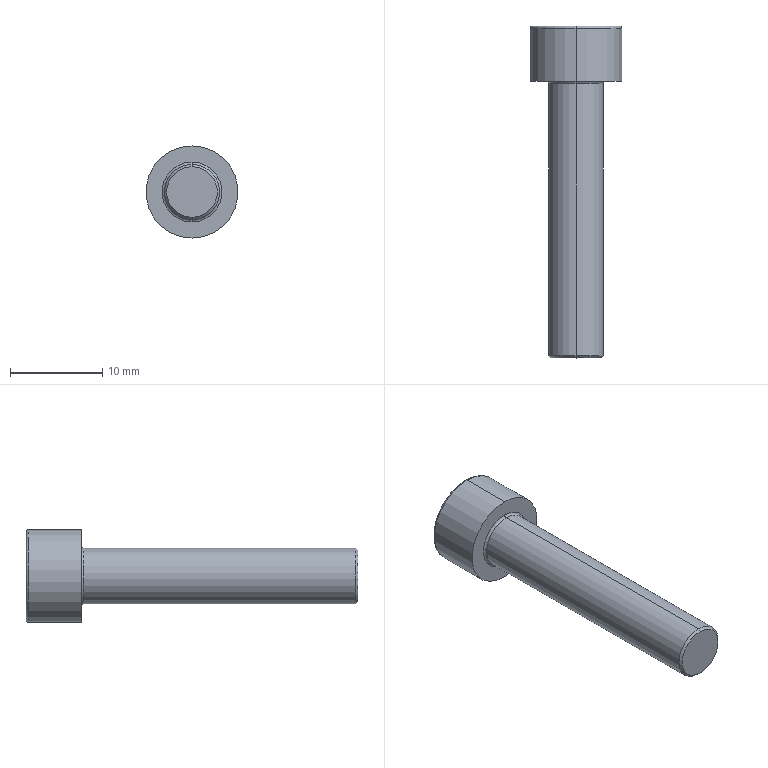Part | STEP file | 1 solid | 20 faces | box 10 x 36 x 10 mm | volume 1254 mm3 | plane 10 | torus 4 | cylinder 4 | cone 2 | commonest cylinder face diameters 6 x2 10 x2
STEP:
#1=CARTESIAN_POINT('',(0.,-30.,-2.75));
#2=VERTEX_POINT('',#1);
#3=CARTESIAN_POINT('',(0.,-30.,2.75));
#4=VERTEX_POINT('',#3);
#5=CARTESIAN_POINT('',(0.,-30.,0.));
#6=DIRECTION('',(0.,-1.,0.));
#7=DIRECTION('',(0.,0.,-1.));
#8=AXIS2_PLACEMENT_3D('',#5,#6,#7);
#9=CIRCLE('',#8,2.75);
#10=EDGE_CURVE('',#2,#4,#9,.T.);
#11=ORIENTED_EDGE('',*,*,#10,.F.);
#12=CARTESIAN_POINT('',(0.,-29.75,-3.));
#13=VERTEX_POINT('',#12);
#14=CARTESIAN_POINT('',(0.,-30.,-2.75));
#15=DIRECTION('',(0.,0.7071,-0.7071));
#16=VECTOR('',#15,1000.);
#17=LINE('',#14,#16);
#18=EDGE_CURVE('',#2,#13,#17,.T.);
#19=ORIENTED_EDGE('',*,*,#18,.T.);
#20=CARTESIAN_POINT('',(0.,-29.75,3.));
#21=VERTEX_POINT('',#20);
#22=CARTESIAN_POINT('',(0.,-29.75,0.));
#23=DIRECTION('',(0.,1.,0.));
#24=DIRECTION('',(0.,0.,-1.));
#25=AXIS2_PLACEMENT_3D('',#22,#23,#24);
#26=CIRCLE('',#25,3.);
#27=EDGE_CURVE('',#21,#13,#26,.T.);
#28=ORIENTED_EDGE('',*,*,#27,.F.);
#29=CARTESIAN_POINT('',(0.,-30.,2.75));
#30=DIRECTION('',(0.,0.7071,0.7071));
#31=VECTOR('',#30,1000.);
#32=LINE('',#29,#31);
#33=EDGE_CURVE('',#4,#21,#32,.T.);
#34=ORIENTED_EDGE('',*,*,#33,.F.);
#35=EDGE_LOOP('',(#11,#19,#28,#34));
#36=FACE_OUTER_BOUND('',#35,.T.);
#37=CARTESIAN_POINT('',(0.,-30.,0.));
#38=DIRECTION('',(0.,1.,0.));
#39=DIRECTION('',(0.,0.,1.));
#40=AXIS2_PLACEMENT_3D('',#37,#38,#39);
#41=CONICAL_SURFACE('',#40,2.75,0.7854);
#42=ADVANCED_FACE('',(#36),#41,.T.);
#43=CARTESIAN_POINT('',(0.,5.75,-5.));
#44=VERTEX_POINT('',#43);
#45=CARTESIAN_POINT('',(0.,5.75,5.));
#46=VERTEX_POINT('',#45);
#47=CARTESIAN_POINT('',(0.,5.75,0.));
#48=DIRECTION('',(0.,-1.,0.));
#49=DIRECTION('',(0.,0.,1.));
#50=AXIS2_PLACEMENT_3D('',#47,#48,#49);
#51=CIRCLE('',#50,5.);
#52=EDGE_CURVE('',#44,#46,#51,.T.);
#53=ORIENTED_EDGE('',*,*,#52,.F.);
#54=CARTESIAN_POINT('',(0.,6.,-4.75));
#55=VERTEX_POINT('',#54);
#56=CARTESIAN_POINT('',(0.,5.75,-4.75));
#57=DIRECTION('',(1.,0.,0.));
#58=DIRECTION('',(0.,0.,-1.));
#59=AXIS2_PLACEMENT_3D('',#56,#57,#58);
#60=CIRCLE('',#59,0.25);
#61=EDGE_CURVE('',#44,#55,#60,.T.);
#62=ORIENTED_EDGE('',*,*,#61,.T.);
#63=CARTESIAN_POINT('',(0.,6.,4.75));
#64=VERTEX_POINT('',#63);
#65=CARTESIAN_POINT('',(0.,6.,0.));
#66=DIRECTION('',(0.,1.,0.));
#67=DIRECTION('',(0.,0.,1.));
#68=AXIS2_PLACEMENT_3D('',#65,#66,#67);
#69=CIRCLE('',#68,4.75);
#70=EDGE_CURVE('',#64,#55,#69,.T.);
#71=ORIENTED_EDGE('',*,*,#70,.F.);
#72=CARTESIAN_POINT('',(0.,5.75,4.75));
#73=DIRECTION('',(-1.,0.,0.));
#74=DIRECTION('',(0.,0.,1.));
#75=AXIS2_PLACEMENT_3D('',#72,#73,#74);
#76=CIRCLE('',#75,0.25);
#77=EDGE_CURVE('',#46,#64,#76,.T.);
#78=ORIENTED_EDGE('',*,*,#77,.F.);
#79=EDGE_LOOP('',(#53,#62,#71,#78));
#80=FACE_OUTER_BOUND('',#79,.T.);
#81=CARTESIAN_POINT('',(0.,5.75,0.));
#82=DIRECTION('',(0.,1.,0.));
#83=DIRECTION('',(0.,0.,1.));
#84=AXIS2_PLACEMENT_3D('',#81,#82,#83);
#85=TOROIDAL_SURFACE('',#84,4.75,0.25);
#86=ADVANCED_FACE('',(#80),#85,.T.);
#87=CARTESIAN_POINT('',(0.,-0.25,3.));
#88=VERTEX_POINT('',#87);
#89=CARTESIAN_POINT('',(0.,-0.25,-3.));
#90=VERTEX_POINT('',#89);
#91=CARTESIAN_POINT('',(0.,-0.25,0.));
#92=DIRECTION('',(0.,-1.,0.));
#93=DIRECTION('',(0.,0.,-1.));
#94=AXIS2_PLACEMENT_3D('',#91,#92,#93);
#95=CIRCLE('',#94,3.);
#96=EDGE_CURVE('',#88,#90,#95,.T.);
#97=ORIENTED_EDGE('',*,*,#96,.F.);
#98=CARTESIAN_POINT('',(0.,0.,3.25));
#99=VERTEX_POINT('',#98);
#100=CARTESIAN_POINT('',(0.,-0.25,3.25));
#101=DIRECTION('',(1.,0.,0.));
#102=DIRECTION('',(0.,0.,-1.));
#103=AXIS2_PLACEMENT_3D('',#100,#101,#102);
#104=CIRCLE('',#103,0.25);
#105=EDGE_CURVE('',#88,#99,#104,.T.);
#106=ORIENTED_EDGE('',*,*,#105,.T.);
#107=CARTESIAN_POINT('',(0.,0.,-3.25));
#108=VERTEX_POINT('',#107);
#109=CARTESIAN_POINT('',(0.,0.,0.));
#110=DIRECTION('',(0.,1.,0.));
#111=DIRECTION('',(0.,0.,-1.));
#112=AXIS2_PLACEMENT_3D('',#109,#110,#111);
#113=CIRCLE('',#112,3.25);
#114=EDGE_CURVE('',#108,#99,#113,.T.);
#115=ORIENTED_EDGE('',*,*,#114,.F.);
#116=CARTESIAN_POINT('',(0.,-0.25,-3.25));
#117=DIRECTION('',(-1.,0.,0.));
#118=DIRECTION('',(0.,0.,1.));
#119=AXIS2_PLACEMENT_3D('',#116,#117,#118);
#120=CIRCLE('',#119,0.25);
#121=EDGE_CURVE('',#90,#108,#120,.T.);
#122=ORIENTED_EDGE('',*,*,#121,.F.);
#123=EDGE_LOOP('',(#97,#106,#115,#122));
#124=FACE_OUTER_BOUND('',#123,.T.);
#125=CARTESIAN_POINT('',(0.,-0.25,0.));
#126=DIRECTION('',(0.,-1.,0.));
#127=DIRECTION('',(0.,0.,-1.));
#128=AXIS2_PLACEMENT_3D('',#125,#126,#127);
#129=TOROIDAL_SURFACE('',#128,3.25,0.25);
#130=ADVANCED_FACE('',(#124),#129,.F.);
#131=CARTESIAN_POINT('',(0.,-0.25,0.));
#132=DIRECTION('',(0.,-1.,0.));
#133=DIRECTION('',(0.,0.,-1.));
#134=AXIS2_PLACEMENT_3D('',#131,#132,#133);
#135=CIRCLE('',#134,3.);
#136=EDGE_CURVE('',#90,#88,#135,.T.);
#137=ORIENTED_EDGE('',*,*,#136,.T.);
#138=CARTESIAN_POINT('',(0.,0.,3.));
#139=DIRECTION('',(0.,-1.,0.));
#140=VECTOR('',#139,1000.);
#141=LINE('',#138,#140);
#142=EDGE_CURVE('',#88,#21,#141,.T.);
#143=ORIENTED_EDGE('',*,*,#142,.T.);
#144=ORIENTED_EDGE('',*,*,#27,.T.);
#145=CARTESIAN_POINT('',(0.,0.,-3.));
#146=DIRECTION('',(0.,-1.,0.));
#147=VECTOR('',#146,1000.);
#148=LINE('',#145,#147);
#149=EDGE_CURVE('',#90,#13,#148,.T.);
#150=ORIENTED_EDGE('',*,*,#149,.F.);
#151=EDGE_LOOP('',(#137,#143,#144,#150));
#152=FACE_OUTER_BOUND('',#151,.T.);
#153=CARTESIAN_POINT('',(0.,0.,0.));
#154=DIRECTION('',(0.,-1.,0.));
#155=DIRECTION('',(0.,0.,-1.));
#156=AXIS2_PLACEMENT_3D('',#153,#154,#155);
#157=CYLINDRICAL_SURFACE('',#156,3.);
#158=ADVANCED_FACE('',(#152),#157,.T.);
#159=ORIENTED_EDGE('',*,*,#52,.T.);
#160=CARTESIAN_POINT('',(0.,0.,5.));
#161=VERTEX_POINT('',#160);
#162=CARTESIAN_POINT('',(0.,0.,5.));
#163=DIRECTION('',(0.,-1.,0.));
#164=VECTOR('',#163,1000.);
#165=LINE('',#162,#164);
#166=EDGE_CURVE('',#46,#161,#165,.T.);
#167=ORIENTED_EDGE('',*,*,#166,.T.);
#168=CARTESIAN_POINT('',(0.,0.,-5.));
#169=VERTEX_POINT('',#168);
#170=CARTESIAN_POINT('',(0.,0.,0.));
#171=DIRECTION('',(0.,-1.,0.));
#172=DIRECTION('',(0.,0.,-1.));
#173=AXIS2_PLACEMENT_3D('',#170,#171,#172);
#174=CIRCLE('',#173,5.);
#175=EDGE_CURVE('',#169,#161,#174,.T.);
#176=ORIENTED_EDGE('',*,*,#175,.F.);
#177=CARTESIAN_POINT('',(0.,0.,-5.));
#178=DIRECTION('',(0.,-1.,0.));
#179=VECTOR('',#178,1000.);
#180=LINE('',#177,#179);
#181=EDGE_CURVE('',#44,#169,#180,.T.);
#182=ORIENTED_EDGE('',*,*,#181,.F.);
#183=EDGE_LOOP('',(#159,#167,#176,#182));
#184=FACE_OUTER_BOUND('',#183,.T.);
#185=CARTESIAN_POINT('',(0.,0.,0.));
#186=DIRECTION('',(0.,-1.,0.));
#187=DIRECTION('',(0.,0.,-1.));
#188=AXIS2_PLACEMENT_3D('',#185,#186,#187);
#189=CYLINDRICAL_SURFACE('',#188,5.);
#190=ADVANCED_FACE('',(#184),#189,.T.);
#191=ORIENTED_EDGE('',*,*,#70,.T.);
#192=CARTESIAN_POINT('',(0.,6.,0.));
#193=DIRECTION('',(0.,1.,0.));
#194=DIRECTION('',(0.,0.,1.));
#195=AXIS2_PLACEMENT_3D('',#192,#193,#194);
#196=CIRCLE('',#195,4.75);
#197=EDGE_CURVE('',#55,#64,#196,.T.);
#198=ORIENTED_EDGE('',*,*,#197,.T.);
#199=EDGE_LOOP('',(#191,#198));
#200=FACE_OUTER_BOUND('',#199,.T.);
#201=CARTESIAN_POINT('',(0.,6.,-2.887));
#202=VERTEX_POINT('',#201);
#203=CARTESIAN_POINT('',(-2.5,6.,-1.443));
#204=VERTEX_POINT('',#203);
#205=CARTESIAN_POINT('',(0.,6.,-2.887));
#206=DIRECTION('',(-0.866,0.,0.5));
#207=VECTOR('',#206,1000.);
#208=LINE('',#205,#207);
#209=EDGE_CURVE('',#202,#204,#208,.T.);
#210=ORIENTED_EDGE('',*,*,#209,.F.);
#211=CARTESIAN_POINT('',(2.5,6.,-1.443));
#212=VERTEX_POINT('',#211);
#213=CARTESIAN_POINT('',(2.5,6.,-1.443));
#214=DIRECTION('',(-0.866,0.,-0.5));
#215=VECTOR('',#214,1000.);
#216=LINE('',#213,#215);
#217=EDGE_CURVE('',#212,#202,#216,.T.);
#218=ORIENTED_EDGE('',*,*,#217,.F.);
#219=CARTESIAN_POINT('',(2.5,6.,1.443));
#220=VERTEX_POINT('',#219);
#221=CARTESIAN_POINT('',(2.5,6.,1.443));
#222=DIRECTION('',(0.,0.,-1.));
#223=VECTOR('',#222,1000.);
#224=LINE('',#221,#223);
#225=EDGE_CURVE('',#220,#212,#224,.T.);
#226=ORIENTED_EDGE('',*,*,#225,.F.);
#227=CARTESIAN_POINT('',(0.,6.,2.887));
#228=VERTEX_POINT('',#227);
#229=CARTESIAN_POINT('',(0.,6.,2.887));
#230=DIRECTION('',(0.866,0.,-0.5));
#231=VECTOR('',#230,1000.);
#232=LINE('',#229,#231);
#233=EDGE_CURVE('',#228,#220,#232,.T.);
#234=ORIENTED_EDGE('',*,*,#233,.F.);
#235=CARTESIAN_POINT('',(-2.5,6.,1.443));
#236=VERTEX_POINT('',#235);
#237=CARTESIAN_POINT('',(-2.5,6.,1.443));
#238=DIRECTION('',(0.866,0.,0.5));
#239=VECTOR('',#238,1000.);
#240=LINE('',#237,#239);
#241=EDGE_CURVE('',#236,#228,#240,.T.);
#242=ORIENTED_EDGE('',*,*,#241,.F.);
#243=CARTESIAN_POINT('',(-2.5,6.,-1.443));
#244=DIRECTION('',(0.,0.,1.));
#245=VECTOR('',#244,1000.);
#246=LINE('',#243,#245);
#247=EDGE_CURVE('',#204,#236,#246,.T.);
#248=ORIENTED_EDGE('',*,*,#247,.F.);
#249=EDGE_LOOP('',(#210,#218,#226,#234,#242,#248));
#250=FACE_BOUND('',#249,.T.);
#251=CARTESIAN_POINT('',(0.,6.,0.));
#252=DIRECTION('',(0.,1.,0.));
#253=DIRECTION('',(0.,0.,1.));
#254=AXIS2_PLACEMENT_3D('',#251,#252,#253);
#255=PLANE('',#254);
#256=ADVANCED_FACE('',(#200,#250),#255,.T.);
#257=ORIENTED_EDGE('',*,*,#166,.F.);
#258=CARTESIAN_POINT('',(0.,5.75,0.));
#259=DIRECTION('',(0.,-1.,0.));
#260=DIRECTION('',(0.,0.,1.));
#261=AXIS2_PLACEMENT_3D('',#258,#259,#260);
#262=CIRCLE('',#261,5.);
#263=EDGE_CURVE('',#46,#44,#262,.T.);
#264=ORIENTED_EDGE('',*,*,#263,.T.);
#265=ORIENTED_EDGE('',*,*,#181,.T.);
#266=CARTESIAN_POINT('',(0.,0.,0.));
#267=DIRECTION('',(0.,-1.,0.));
#268=DIRECTION('',(0.,0.,-1.));
#269=AXIS2_PLACEMENT_3D('',#266,#267,#268);
#270=CIRCLE('',#269,5.);
#271=EDGE_CURVE('',#161,#169,#270,.T.);
#272=ORIENTED_EDGE('',*,*,#271,.F.);
#273=EDGE_LOOP('',(#257,#264,#265,#272));
#274=FACE_OUTER_BOUND('',#273,.T.);
#275=CARTESIAN_POINT('',(0.,0.,0.));
#276=DIRECTION('',(0.,-1.,0.));
#277=DIRECTION('',(0.,0.,-1.));
#278=AXIS2_PLACEMENT_3D('',#275,#276,#277);
#279=CYLINDRICAL_SURFACE('',#278,5.);
#280=ADVANCED_FACE('',(#274),#279,.T.);
#281=ORIENTED_EDGE('',*,*,#114,.T.);
#282=CARTESIAN_POINT('',(0.,0.,0.));
#283=DIRECTION('',(0.,1.,0.));
#284=DIRECTION('',(0.,0.,-1.));
#285=AXIS2_PLACEMENT_3D('',#282,#283,#284);
#286=CIRCLE('',#285,3.25);
#287=EDGE_CURVE('',#99,#108,#286,.T.);
#288=ORIENTED_EDGE('',*,*,#287,.T.);
#289=EDGE_LOOP('',(#281,#288));
#290=FACE_BOUND('',#289,.T.);
#291=ORIENTED_EDGE('',*,*,#175,.T.);
#292=ORIENTED_EDGE('',*,*,#271,.T.);
#293=EDGE_LOOP('',(#291,#292));
#294=FACE_OUTER_BOUND('',#293,.T.);
#295=CARTESIAN_POINT('',(5.,0.,0.));
#296=DIRECTION('',(0.,-1.,0.));
#297=DIRECTION('',(0.,0.,-1.));
#298=AXIS2_PLACEMENT_3D('',#295,#296,#297);
#299=PLANE('',#298);
#300=ADVANCED_FACE('',(#290,#294),#299,.T.);
#301=ORIENTED_EDGE('',*,*,#142,.F.);
#302=ORIENTED_EDGE('',*,*,#96,.T.);
#303=ORIENTED_EDGE('',*,*,#149,.T.);
#304=CARTESIAN_POINT('',(0.,-29.75,0.));
#305=DIRECTION('',(0.,1.,0.));
#306=DIRECTION('',(0.,0.,-1.));
#307=AXIS2_PLACEMENT_3D('',#304,#305,#306);
#308=CIRCLE('',#307,3.);
#309=EDGE_CURVE('',#13,#21,#308,.T.);
#310=ORIENTED_EDGE('',*,*,#309,.T.);
#311=EDGE_LOOP('',(#301,#302,#303,#310));
#312=FACE_OUTER_BOUND('',#311,.T.);
#313=CARTESIAN_POINT('',(0.,0.,0.));
#314=DIRECTION('',(0.,-1.,0.));
#315=DIRECTION('',(0.,0.,-1.));
#316=AXIS2_PLACEMENT_3D('',#313,#314,#315);
#317=CYLINDRICAL_SURFACE('',#316,3.);
#318=ADVANCED_FACE('',(#312),#317,.T.);
#319=CARTESIAN_POINT('',(0.,-30.,0.));
#320=DIRECTION('',(0.,-1.,0.));
#321=DIRECTION('',(0.,0.,-1.));
#322=AXIS2_PLACEMENT_3D('',#319,#320,#321);
#323=CIRCLE('',#322,2.75);
#324=EDGE_CURVE('',#4,#2,#323,.T.);
#325=ORIENTED_EDGE('',*,*,#324,.T.);
#326=ORIENTED_EDGE('',*,*,#10,.T.);
#327=EDGE_LOOP('',(#325,#326));
#328=FACE_OUTER_BOUND('',#327,.T.);
#329=CARTESIAN_POINT('',(3.,-30.,0.));
#330=DIRECTION('',(0.,-1.,0.));
#331=DIRECTION('',(0.,0.,-1.));
#332=AXIS2_PLACEMENT_3D('',#329,#330,#331);
#333=PLANE('',#332);
#334=ADVANCED_FACE('',(#328),#333,.T.);
#335=ORIENTED_EDGE('',*,*,#209,.T.);
#336=CARTESIAN_POINT('',(-2.5,3.,-1.443));
#337=VERTEX_POINT('',#336);
#338=CARTESIAN_POINT('',(-2.5,3.,-1.443));
#339=DIRECTION('',(0.,1.,0.));
#340=VECTOR('',#339,1000.);
#341=LINE('',#338,#340);
#342=EDGE_CURVE('',#337,#204,#341,.T.);
#343=ORIENTED_EDGE('',*,*,#342,.F.);
#344=CARTESIAN_POINT('',(0.,3.,-2.887));
#345=VERTEX_POINT('',#344);
#346=CARTESIAN_POINT('',(0.,3.,-2.887));
#347=DIRECTION('',(-0.866,0.,0.5));
#348=VECTOR('',#347,1000.);
#349=LINE('',#346,#348);
#350=EDGE_CURVE('',#345,#337,#349,.T.);
#351=ORIENTED_EDGE('',*,*,#350,.F.);
#352=CARTESIAN_POINT('',(0.,3.,-2.887));
#353=DIRECTION('',(0.,1.,0.));
#354=VECTOR('',#353,1000.);
#355=LINE('',#352,#354);
#356=EDGE_CURVE('',#345,#202,#355,.T.);
#357=ORIENTED_EDGE('',*,*,#356,.T.);
#358=EDGE_LOOP('',(#335,#343,#351,#357));
#359=FACE_OUTER_BOUND('',#358,.T.);
#360=CARTESIAN_POINT('',(0.,3.,-2.887));
#361=DIRECTION('',(-0.5,0.,-0.866));
#362=DIRECTION('',(-0.866,0.,0.5));
#363=AXIS2_PLACEMENT_3D('',#360,#361,#362);
#364=PLANE('',#363);
#365=ADVANCED_FACE('',(#359),#364,.F.);
#366=ORIENTED_EDGE('',*,*,#217,.T.);
#367=ORIENTED_EDGE('',*,*,#356,.F.);
#368=CARTESIAN_POINT('',(2.5,3.,-1.443));
#369=VERTEX_POINT('',#368);
#370=CARTESIAN_POINT('',(2.5,3.,-1.443));
#371=DIRECTION('',(-0.866,0.,-0.5));
#372=VECTOR('',#371,1000.);
#373=LINE('',#370,#372);
#374=EDGE_CURVE('',#369,#345,#373,.T.);
#375=ORIENTED_EDGE('',*,*,#374,.F.);
#376=CARTESIAN_POINT('',(2.5,3.,-1.443));
#377=DIRECTION('',(0.,1.,0.));
#378=VECTOR('',#377,1000.);
#379=LINE('',#376,#378);
#380=EDGE_CURVE('',#369,#212,#379,.T.);
#381=ORIENTED_EDGE('',*,*,#380,.T.);
#382=EDGE_LOOP('',(#366,#367,#375,#381));
#383=FACE_OUTER_BOUND('',#382,.T.);
#384=CARTESIAN_POINT('',(2.5,3.,-1.443));
#385=DIRECTION('',(0.5,0.,-0.866));
#386=DIRECTION('',(-0.866,0.,-0.5));
#387=AXIS2_PLACEMENT_3D('',#384,#385,#386);
#388=PLANE('',#387);
#389=ADVANCED_FACE('',(#383),#388,.F.);
#390=ORIENTED_EDGE('',*,*,#225,.T.);
#391=ORIENTED_EDGE('',*,*,#380,.F.);
#392=CARTESIAN_POINT('',(2.5,3.,1.443));
#393=VERTEX_POINT('',#392);
#394=CARTESIAN_POINT('',(2.5,3.,1.443));
#395=DIRECTION('',(0.,0.,-1.));
#396=VECTOR('',#395,1000.);
#397=LINE('',#394,#396);
#398=EDGE_CURVE('',#393,#369,#397,.T.);
#399=ORIENTED_EDGE('',*,*,#398,.F.);
#400=CARTESIAN_POINT('',(2.5,3.,1.443));
#401=DIRECTION('',(0.,1.,0.));
#402=VECTOR('',#401,1000.);
#403=LINE('',#400,#402);
#404=EDGE_CURVE('',#393,#220,#403,.T.);
#405=ORIENTED_EDGE('',*,*,#404,.T.);
#406=EDGE_LOOP('',(#390,#391,#399,#405));
#407=FACE_OUTER_BOUND('',#406,.T.);
#408=CARTESIAN_POINT('',(2.5,3.,1.443));
#409=DIRECTION('',(1.,0.,0.));
#410=DIRECTION('',(0.,0.,-1.));
#411=AXIS2_PLACEMENT_3D('',#408,#409,#410);
#412=PLANE('',#411);
#413=ADVANCED_FACE('',(#407),#412,.F.);
#414=ORIENTED_EDGE('',*,*,#233,.T.);
#415=ORIENTED_EDGE('',*,*,#404,.F.);
#416=CARTESIAN_POINT('',(0.,3.,2.887));
#417=VERTEX_POINT('',#416);
#418=CARTESIAN_POINT('',(0.,3.,2.887));
#419=DIRECTION('',(0.866,0.,-0.5));
#420=VECTOR('',#419,1000.);
#421=LINE('',#418,#420);
#422=EDGE_CURVE('',#417,#393,#421,.T.);
#423=ORIENTED_EDGE('',*,*,#422,.F.);
#424=CARTESIAN_POINT('',(0.,3.,2.887));
#425=DIRECTION('',(0.,1.,0.));
#426=VECTOR('',#425,1000.);
#427=LINE('',#424,#426);
#428=EDGE_CURVE('',#417,#228,#427,.T.);
#429=ORIENTED_EDGE('',*,*,#428,.T.);
#430=EDGE_LOOP('',(#414,#415,#423,#429));
#431=FACE_OUTER_BOUND('',#430,.T.);
#432=CARTESIAN_POINT('',(0.,3.,2.887));
#433=DIRECTION('',(0.5,0.,0.866));
#434=DIRECTION('',(0.866,0.,-0.5));
#435=AXIS2_PLACEMENT_3D('',#432,#433,#434);
#436=PLANE('',#435);
#437=ADVANCED_FACE('',(#431),#436,.F.);
#438=ORIENTED_EDGE('',*,*,#241,.T.);
#439=ORIENTED_EDGE('',*,*,#428,.F.);
#440=CARTESIAN_POINT('',(-2.5,3.,1.443));
#441=VERTEX_POINT('',#440);
#442=CARTESIAN_POINT('',(-2.5,3.,1.443));
#443=DIRECTION('',(0.866,0.,0.5));
#444=VECTOR('',#443,1000.);
#445=LINE('',#442,#444);
#446=EDGE_CURVE('',#441,#417,#445,.T.);
#447=ORIENTED_EDGE('',*,*,#446,.F.);
#448=CARTESIAN_POINT('',(-2.5,3.,1.443));
#449=DIRECTION('',(0.,1.,0.));
#450=VECTOR('',#449,1000.);
#451=LINE('',#448,#450);
#452=EDGE_CURVE('',#441,#236,#451,.T.);
#453=ORIENTED_EDGE('',*,*,#452,.T.);
#454=EDGE_LOOP('',(#438,#439,#447,#453));
#455=FACE_OUTER_BOUND('',#454,.T.);
#456=CARTESIAN_POINT('',(-2.5,3.,1.443));
#457=DIRECTION('',(-0.5,0.,0.866));
#458=DIRECTION('',(0.866,0.,0.5));
#459=AXIS2_PLACEMENT_3D('',#456,#457,#458);
#460=PLANE('',#459);
#461=ADVANCED_FACE('',(#455),#460,.F.);
#462=ORIENTED_EDGE('',*,*,#247,.T.);
#463=ORIENTED_EDGE('',*,*,#452,.F.);
#464=CARTESIAN_POINT('',(-2.5,3.,-1.443));
#465=DIRECTION('',(0.,0.,1.));
#466=VECTOR('',#465,1000.);
#467=LINE('',#464,#466);
#468=EDGE_CURVE('',#337,#441,#467,.T.);
#469=ORIENTED_EDGE('',*,*,#468,.F.);
#470=ORIENTED_EDGE('',*,*,#342,.T.);
#471=EDGE_LOOP('',(#462,#463,#469,#470));
#472=FACE_OUTER_BOUND('',#471,.T.);
#473=CARTESIAN_POINT('',(-2.5,3.,-1.443));
#474=DIRECTION('',(-1.,0.,0.));
#475=DIRECTION('',(0.,0.,1.));
#476=AXIS2_PLACEMENT_3D('',#473,#474,#475);
#477=PLANE('',#476);
#478=ADVANCED_FACE('',(#472),#477,.F.);
#479=ORIENTED_EDGE('',*,*,#350,.T.);
#480=ORIENTED_EDGE('',*,*,#468,.T.);
#481=ORIENTED_EDGE('',*,*,#446,.T.);
#482=ORIENTED_EDGE('',*,*,#422,.T.);
#483=ORIENTED_EDGE('',*,*,#398,.T.);
#484=ORIENTED_EDGE('',*,*,#374,.T.);
#485=EDGE_LOOP('',(#479,#480,#481,#482,#483,#484));
#486=FACE_OUTER_BOUND('',#485,.T.);
#487=CARTESIAN_POINT('',(0.,3.,0.));
#488=DIRECTION('',(0.,1.,0.));
#489=DIRECTION('',(0.,0.,1.));
#490=AXIS2_PLACEMENT_3D('',#487,#488,#489);
#491=PLANE('',#490);
#492=ADVANCED_FACE('',(#486),#491,.T.);
#493=ORIENTED_EDGE('',*,*,#105,.F.);
#494=ORIENTED_EDGE('',*,*,#136,.F.);
#495=ORIENTED_EDGE('',*,*,#121,.T.);
#496=ORIENTED_EDGE('',*,*,#287,.F.);
#497=EDGE_LOOP('',(#493,#494,#495,#496));
#498=FACE_OUTER_BOUND('',#497,.T.);
#499=CARTESIAN_POINT('',(0.,-0.25,0.));
#500=DIRECTION('',(0.,-1.,0.));
#501=DIRECTION('',(0.,0.,-1.));
#502=AXIS2_PLACEMENT_3D('',#499,#500,#501);
#503=TOROIDAL_SURFACE('',#502,3.25,0.25);
#504=ADVANCED_FACE('',(#498),#503,.F.);
#505=ORIENTED_EDGE('',*,*,#61,.F.);
#506=ORIENTED_EDGE('',*,*,#263,.F.);
#507=ORIENTED_EDGE('',*,*,#77,.T.);
#508=ORIENTED_EDGE('',*,*,#197,.F.);
#509=EDGE_LOOP('',(#505,#506,#507,#508));
#510=FACE_OUTER_BOUND('',#509,.T.);
#511=CARTESIAN_POINT('',(0.,5.75,0.));
#512=DIRECTION('',(0.,1.,0.));
#513=DIRECTION('',(0.,0.,1.));
#514=AXIS2_PLACEMENT_3D('',#511,#512,#513);
#515=TOROIDAL_SURFACE('',#514,4.75,0.25);
#516=ADVANCED_FACE('',(#510),#515,.T.);
#517=ORIENTED_EDGE('',*,*,#18,.F.);
#518=ORIENTED_EDGE('',*,*,#324,.F.);
#519=ORIENTED_EDGE('',*,*,#33,.T.);
#520=ORIENTED_EDGE('',*,*,#309,.F.);
#521=EDGE_LOOP('',(#517,#518,#519,#520));
#522=FACE_OUTER_BOUND('',#521,.T.);
#523=CARTESIAN_POINT('',(0.,-30.,0.));
#524=DIRECTION('',(0.,1.,0.));
#525=DIRECTION('',(0.,0.,1.));
#526=AXIS2_PLACEMENT_3D('',#523,#524,#525);
#527=CONICAL_SURFACE('',#526,2.75,0.7854);
#528=ADVANCED_FACE('',(#522),#527,.T.);
#529=CLOSED_SHELL('',(#42,#86,#130,#158,#190,#256,#280,#300,#318,#334,#365,#389,#413,#437,#461,#478,#492,#504,#516,#528));
#530=MANIFOLD_SOLID_BREP('',#529);
#531=CARTESIAN_POINT('',(0.,0.,0.));
#532=DIRECTION('',(0.,0.,1.));
#533=DIRECTION('',(1.,0.,0.));
#534=AXIS2_PLACEMENT_3D('',#531,#532,#533);
#535=(LENGTH_UNIT()NAMED_UNIT(*)SI_UNIT(.MILLI.,.METRE.));
#536=UNCERTAINTY_MEASURE_WITH_UNIT(LENGTH_MEASURE(0.00001),#535,'','');
#537=(NAMED_UNIT(*)PLANE_ANGLE_UNIT()SI_UNIT($,.RADIAN.));
#538=(NAMED_UNIT(*)SI_UNIT($,.STERADIAN.)SOLID_ANGLE_UNIT());
#539=(GEOMETRIC_REPRESENTATION_CONTEXT(3)GLOBAL_UNCERTAINTY_ASSIGNED_CONTEXT((#536))GLOBAL_UNIT_ASSIGNED_CONTEXT((#535,#537,#538))REPRESENTATION_CONTEXT('',''));
#540=ADVANCED_BREP_SHAPE_REPRESENTATION('',(#530,#534),#539);